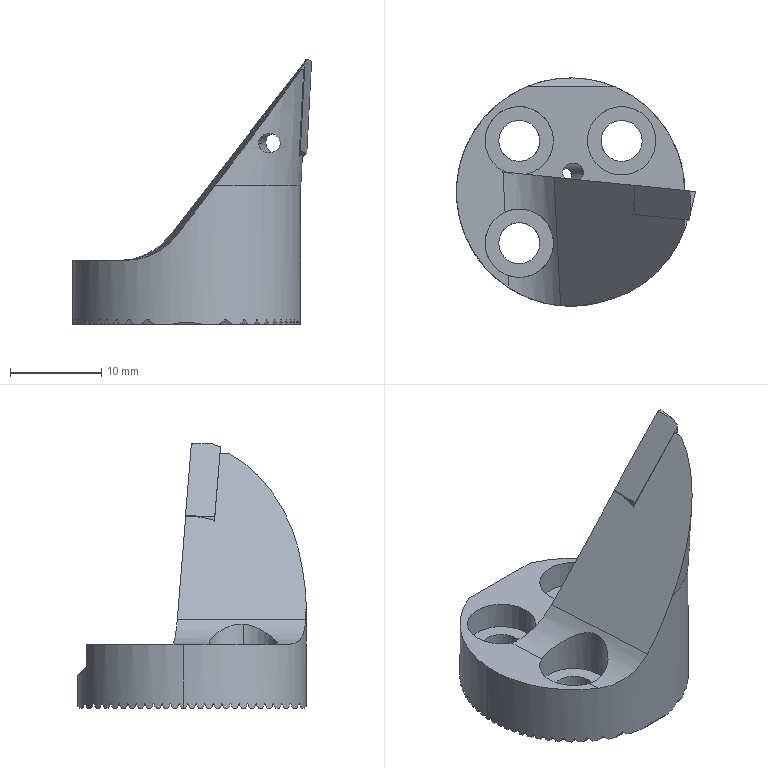Part | 2 solids | 195 faces | volume 4248 mm3 | plane 163 | cylinder 29 | cone 3 | commonest cylinder face diameters 4.5 x6 7.5 x6 0.4 x2 2 x2 2.1 x2 2.8 x2